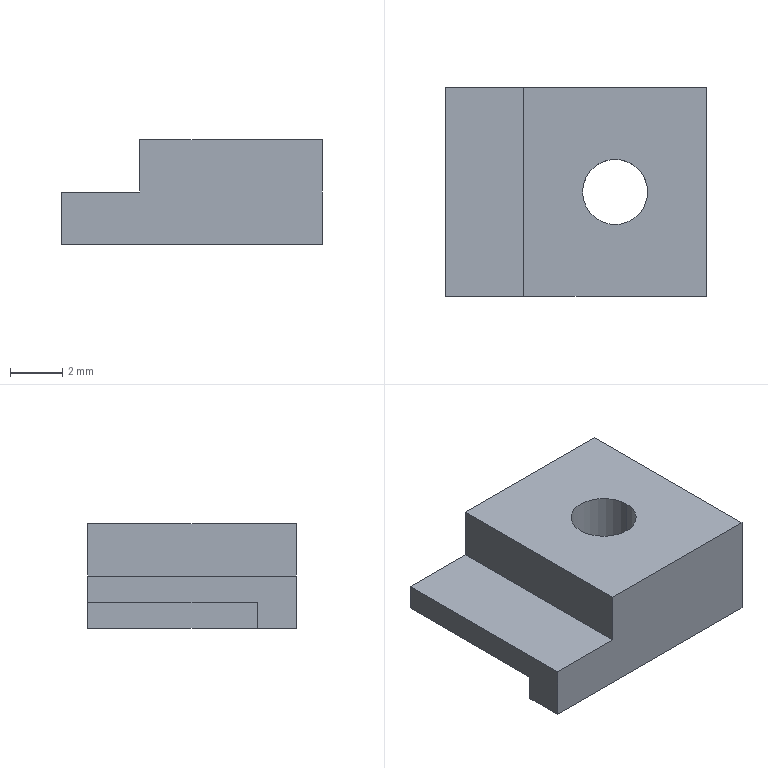Part | SolidWorks | features ICE 4, Extrusion 1, HoleWzd 1, MoveFace 1 | 1 solid | 13 faces | box 10 x 8 x 4 mm | volume 226.365 mm3 | plane 11 | cylinder 2 | commonest cylinder face diameters 2.5 x2
STEP:
#1=CARTESIAN_POINT('',(7.25,-4.,0.));
#2=VERTEX_POINT('',#1);
#3=CARTESIAN_POINT('',(9.75,-4.,0.));
#4=VERTEX_POINT('',#3);
#5=CARTESIAN_POINT('',(8.5,-4.,0.));
#6=DIRECTION('',(0.,0.,1.));
#7=DIRECTION('',(1.,0.,0.));
#8=AXIS2_PLACEMENT_3D('',#5,#6,#7);
#9=CIRCLE('',#8,1.25);
#10=EDGE_CURVE('',#2,#4,#9,.T.);
#11=ORIENTED_EDGE('',*,*,#10,.F.);
#12=CARTESIAN_POINT('',(7.25,-4.,4.));
#13=VERTEX_POINT('',#12);
#14=CARTESIAN_POINT('',(7.25,-4.,4.));
#15=DIRECTION('',(0.,0.,1.));
#16=VECTOR('',#15,1000.);
#17=LINE('',#14,#16);
#18=EDGE_CURVE('',#2,#13,#17,.T.);
#19=ORIENTED_EDGE('',*,*,#18,.T.);
#20=CARTESIAN_POINT('',(9.75,-4.,4.));
#21=VERTEX_POINT('',#20);
#22=CARTESIAN_POINT('',(8.5,-4.,4.));
#23=DIRECTION('',(0.,0.,1.));
#24=DIRECTION('',(1.,0.,0.));
#25=AXIS2_PLACEMENT_3D('',#22,#23,#24);
#26=CIRCLE('',#25,1.25);
#27=EDGE_CURVE('',#13,#21,#26,.T.);
#28=ORIENTED_EDGE('',*,*,#27,.T.);
#29=CARTESIAN_POINT('',(9.75,-4.,4.));
#30=DIRECTION('',(0.,0.,1.));
#31=VECTOR('',#30,1000.);
#32=LINE('',#29,#31);
#33=EDGE_CURVE('',#4,#21,#32,.T.);
#34=ORIENTED_EDGE('',*,*,#33,.F.);
#35=EDGE_LOOP('',(#11,#19,#28,#34));
#36=FACE_OUTER_BOUND('',#35,.T.);
#37=CARTESIAN_POINT('',(8.5,-4.,4.));
#38=DIRECTION('',(0.,0.,1.));
#39=DIRECTION('',(1.,0.,0.));
#40=AXIS2_PLACEMENT_3D('',#37,#38,#39);
#41=CYLINDRICAL_SURFACE('',#40,1.25);
#42=ADVANCED_FACE('',(#36),#41,.F.);
#43=CARTESIAN_POINT('',(2.,-8.,2.));
#44=VERTEX_POINT('',#43);
#45=CARTESIAN_POINT('',(5.,-8.,2.));
#46=VERTEX_POINT('',#45);
#47=CARTESIAN_POINT('',(0.,-8.,2.));
#48=DIRECTION('',(1.,0.,0.));
#49=VECTOR('',#48,1000.);
#50=LINE('',#47,#49);
#51=EDGE_CURVE('',#44,#46,#50,.T.);
#52=ORIENTED_EDGE('',*,*,#51,.F.);
#53=CARTESIAN_POINT('',(2.,-8.,0.));
#54=VERTEX_POINT('',#53);
#55=CARTESIAN_POINT('',(2.,-8.,7.));
#56=DIRECTION('',(0.,0.,-1.));
#57=VECTOR('',#56,1000.);
#58=LINE('',#55,#57);
#59=EDGE_CURVE('',#44,#54,#58,.T.);
#60=ORIENTED_EDGE('',*,*,#59,.T.);
#61=CARTESIAN_POINT('',(12.,-8.,0.));
#62=VERTEX_POINT('',#61);
#63=CARTESIAN_POINT('',(0.,-8.,0.));
#64=DIRECTION('',(1.,0.,0.));
#65=VECTOR('',#64,1000.);
#66=LINE('',#63,#65);
#67=EDGE_CURVE('',#54,#62,#66,.T.);
#68=ORIENTED_EDGE('',*,*,#67,.T.);
#69=CARTESIAN_POINT('',(12.,-8.,4.));
#70=VERTEX_POINT('',#69);
#71=CARTESIAN_POINT('',(12.,-8.,2.));
#72=DIRECTION('',(0.,0.,-1.));
#73=VECTOR('',#72,1000.);
#74=LINE('',#71,#73);
#75=EDGE_CURVE('',#70,#62,#74,.T.);
#76=ORIENTED_EDGE('',*,*,#75,.F.);
#77=CARTESIAN_POINT('',(5.,-8.,4.));
#78=VERTEX_POINT('',#77);
#79=CARTESIAN_POINT('',(12.,-8.,4.));
#80=DIRECTION('',(1.,0.,0.));
#81=VECTOR('',#80,1000.);
#82=LINE('',#79,#81);
#83=EDGE_CURVE('',#78,#70,#82,.T.);
#84=ORIENTED_EDGE('',*,*,#83,.F.);
#85=CARTESIAN_POINT('',(5.,-8.,4.));
#86=DIRECTION('',(0.,0.,-1.));
#87=VECTOR('',#86,1000.);
#88=LINE('',#85,#87);
#89=EDGE_CURVE('',#78,#46,#88,.T.);
#90=ORIENTED_EDGE('',*,*,#89,.T.);
#91=EDGE_LOOP('',(#52,#60,#68,#76,#84,#90));
#92=FACE_OUTER_BOUND('',#91,.T.);
#93=CARTESIAN_POINT('',(0.,-8.,2.));
#94=DIRECTION('',(0.,1.,0.));
#95=DIRECTION('',(0.,0.,1.));
#96=AXIS2_PLACEMENT_3D('',#93,#94,#95);
#97=PLANE('',#96);
#98=ADVANCED_FACE('',(#92),#97,.F.);
#99=CARTESIAN_POINT('',(12.,0.,0.));
#100=VERTEX_POINT('',#99);
#101=CARTESIAN_POINT('',(12.,0.,0.));
#102=DIRECTION('',(0.,1.,0.));
#103=VECTOR('',#102,1000.);
#104=LINE('',#101,#103);
#105=EDGE_CURVE('',#62,#100,#104,.T.);
#106=ORIENTED_EDGE('',*,*,#105,.T.);
#107=CARTESIAN_POINT('',(12.,0.,4.));
#108=VERTEX_POINT('',#107);
#109=CARTESIAN_POINT('',(12.,0.,2.));
#110=DIRECTION('',(0.,0.,-1.));
#111=VECTOR('',#110,1000.);
#112=LINE('',#109,#111);
#113=EDGE_CURVE('',#108,#100,#112,.T.);
#114=ORIENTED_EDGE('',*,*,#113,.F.);
#115=CARTESIAN_POINT('',(12.,-8.,4.));
#116=DIRECTION('',(0.,1.,0.));
#117=VECTOR('',#116,1000.);
#118=LINE('',#115,#117);
#119=EDGE_CURVE('',#70,#108,#118,.T.);
#120=ORIENTED_EDGE('',*,*,#119,.F.);
#121=ORIENTED_EDGE('',*,*,#75,.T.);
#122=EDGE_LOOP('',(#106,#114,#120,#121));
#123=FACE_OUTER_BOUND('',#122,.T.);
#124=CARTESIAN_POINT('',(12.,0.,2.));
#125=DIRECTION('',(-1.,0.,0.));
#126=DIRECTION('',(0.,-1.,0.));
#127=AXIS2_PLACEMENT_3D('',#124,#125,#126);
#128=PLANE('',#127);
#129=ADVANCED_FACE('',(#123),#128,.F.);
#130=CARTESIAN_POINT('',(2.,0.,1.));
#131=VERTEX_POINT('',#130);
#132=CARTESIAN_POINT('',(6.,0.,1.));
#133=VERTEX_POINT('',#132);
#134=CARTESIAN_POINT('',(0.,0.,1.));
#135=DIRECTION('',(1.,0.,0.));
#136=VECTOR('',#135,1000.);
#137=LINE('',#134,#136);
#138=EDGE_CURVE('',#131,#133,#137,.T.);
#139=ORIENTED_EDGE('',*,*,#138,.F.);
#140=CARTESIAN_POINT('',(2.,0.,2.));
#141=VERTEX_POINT('',#140);
#142=CARTESIAN_POINT('',(2.,0.,7.));
#143=DIRECTION('',(0.,0.,-1.));
#144=VECTOR('',#143,1000.);
#145=LINE('',#142,#144);
#146=EDGE_CURVE('',#141,#131,#145,.T.);
#147=ORIENTED_EDGE('',*,*,#146,.F.);
#148=CARTESIAN_POINT('',(5.,0.,2.));
#149=VERTEX_POINT('',#148);
#150=CARTESIAN_POINT('',(0.,0.,2.));
#151=DIRECTION('',(-1.,0.,0.));
#152=VECTOR('',#151,1000.);
#153=LINE('',#150,#152);
#154=EDGE_CURVE('',#149,#141,#153,.T.);
#155=ORIENTED_EDGE('',*,*,#154,.F.);
#156=CARTESIAN_POINT('',(5.,0.,4.));
#157=VERTEX_POINT('',#156);
#158=CARTESIAN_POINT('',(5.,0.,4.));
#159=DIRECTION('',(0.,0.,-1.));
#160=VECTOR('',#159,1000.);
#161=LINE('',#158,#160);
#162=EDGE_CURVE('',#157,#149,#161,.T.);
#163=ORIENTED_EDGE('',*,*,#162,.F.);
#164=CARTESIAN_POINT('',(12.,0.,4.));
#165=DIRECTION('',(-1.,0.,0.));
#166=VECTOR('',#165,1000.);
#167=LINE('',#164,#166);
#168=EDGE_CURVE('',#108,#157,#167,.T.);
#169=ORIENTED_EDGE('',*,*,#168,.F.);
#170=ORIENTED_EDGE('',*,*,#113,.T.);
#171=CARTESIAN_POINT('',(6.,0.,0.));
#172=VERTEX_POINT('',#171);
#173=CARTESIAN_POINT('',(0.,0.,0.));
#174=DIRECTION('',(-1.,0.,0.));
#175=VECTOR('',#174,1000.);
#176=LINE('',#173,#175);
#177=EDGE_CURVE('',#100,#172,#176,.T.);
#178=ORIENTED_EDGE('',*,*,#177,.T.);
#179=CARTESIAN_POINT('',(6.,0.,2.));
#180=DIRECTION('',(0.,0.,1.));
#181=VECTOR('',#180,1000.);
#182=LINE('',#179,#181);
#183=EDGE_CURVE('',#172,#133,#182,.T.);
#184=ORIENTED_EDGE('',*,*,#183,.T.);
#185=EDGE_LOOP('',(#139,#147,#155,#163,#169,#170,#178,#184));
#186=FACE_OUTER_BOUND('',#185,.T.);
#187=CARTESIAN_POINT('',(0.,0.,2.));
#188=DIRECTION('',(0.,-1.,0.));
#189=DIRECTION('',(0.,0.,-1.));
#190=AXIS2_PLACEMENT_3D('',#187,#188,#189);
#191=PLANE('',#190);
#192=ADVANCED_FACE('',(#186),#191,.F.);
#193=CARTESIAN_POINT('',(2.,0.,2.));
#194=DIRECTION('',(0.,1.,0.));
#195=VECTOR('',#194,1000.);
#196=LINE('',#193,#195);
#197=EDGE_CURVE('',#44,#141,#196,.T.);
#198=ORIENTED_EDGE('',*,*,#197,.F.);
#199=ORIENTED_EDGE('',*,*,#51,.T.);
#200=CARTESIAN_POINT('',(5.,-8.,2.));
#201=DIRECTION('',(0.,-1.,0.));
#202=VECTOR('',#201,1000.);
#203=LINE('',#200,#202);
#204=EDGE_CURVE('',#149,#46,#203,.T.);
#205=ORIENTED_EDGE('',*,*,#204,.F.);
#206=ORIENTED_EDGE('',*,*,#154,.T.);
#207=EDGE_LOOP('',(#198,#199,#205,#206));
#208=FACE_OUTER_BOUND('',#207,.T.);
#209=CARTESIAN_POINT('',(0.,0.,2.));
#210=DIRECTION('',(0.,0.,1.));
#211=DIRECTION('',(1.,0.,0.));
#212=AXIS2_PLACEMENT_3D('',#209,#210,#211);
#213=PLANE('',#212);
#214=ADVANCED_FACE('',(#208),#213,.T.);
#215=CARTESIAN_POINT('',(8.5,-4.,0.));
#216=DIRECTION('',(0.,0.,1.));
#217=DIRECTION('',(1.,0.,0.));
#218=AXIS2_PLACEMENT_3D('',#215,#216,#217);
#219=CIRCLE('',#218,1.25);
#220=EDGE_CURVE('',#4,#2,#219,.T.);
#221=ORIENTED_EDGE('',*,*,#220,.T.);
#222=ORIENTED_EDGE('',*,*,#10,.T.);
#223=EDGE_LOOP('',(#221,#222));
#224=FACE_BOUND('',#223,.T.);
#225=ORIENTED_EDGE('',*,*,#67,.F.);
#226=CARTESIAN_POINT('',(2.,-6.5,0.));
#227=VERTEX_POINT('',#226);
#228=CARTESIAN_POINT('',(2.,-8.,0.));
#229=DIRECTION('',(0.,-1.,0.));
#230=VECTOR('',#229,1000.);
#231=LINE('',#228,#230);
#232=EDGE_CURVE('',#227,#54,#231,.T.);
#233=ORIENTED_EDGE('',*,*,#232,.F.);
#234=CARTESIAN_POINT('',(6.,-6.5,0.));
#235=VERTEX_POINT('',#234);
#236=CARTESIAN_POINT('',(6.,-6.5,0.));
#237=DIRECTION('',(-1.,0.,0.));
#238=VECTOR('',#237,1000.);
#239=LINE('',#236,#238);
#240=EDGE_CURVE('',#235,#227,#239,.T.);
#241=ORIENTED_EDGE('',*,*,#240,.F.);
#242=CARTESIAN_POINT('',(6.,0.,0.));
#243=DIRECTION('',(0.,1.,0.));
#244=VECTOR('',#243,1000.);
#245=LINE('',#242,#244);
#246=EDGE_CURVE('',#235,#172,#245,.T.);
#247=ORIENTED_EDGE('',*,*,#246,.T.);
#248=ORIENTED_EDGE('',*,*,#177,.F.);
#249=ORIENTED_EDGE('',*,*,#105,.F.);
#250=EDGE_LOOP('',(#225,#233,#241,#247,#248,#249));
#251=FACE_OUTER_BOUND('',#250,.T.);
#252=CARTESIAN_POINT('',(0.,0.,0.));
#253=DIRECTION('',(0.,0.,1.));
#254=DIRECTION('',(1.,0.,0.));
#255=AXIS2_PLACEMENT_3D('',#252,#253,#254);
#256=PLANE('',#255);
#257=ADVANCED_FACE('',(#224,#251),#256,.F.);
#258=ORIENTED_EDGE('',*,*,#204,.T.);
#259=ORIENTED_EDGE('',*,*,#89,.F.);
#260=CARTESIAN_POINT('',(5.,-8.,4.));
#261=DIRECTION('',(0.,-1.,0.));
#262=VECTOR('',#261,1000.);
#263=LINE('',#260,#262);
#264=EDGE_CURVE('',#157,#78,#263,.T.);
#265=ORIENTED_EDGE('',*,*,#264,.F.);
#266=ORIENTED_EDGE('',*,*,#162,.T.);
#267=EDGE_LOOP('',(#258,#259,#265,#266));
#268=FACE_OUTER_BOUND('',#267,.T.);
#269=CARTESIAN_POINT('',(5.,-8.,4.));
#270=DIRECTION('',(1.,0.,0.));
#271=DIRECTION('',(0.,0.,-1.));
#272=AXIS2_PLACEMENT_3D('',#269,#270,#271);
#273=PLANE('',#272);
#274=ADVANCED_FACE('',(#268),#273,.F.);
#275=CARTESIAN_POINT('',(8.5,-4.,4.));
#276=DIRECTION('',(0.,0.,1.));
#277=DIRECTION('',(1.,0.,0.));
#278=AXIS2_PLACEMENT_3D('',#275,#276,#277);
#279=CIRCLE('',#278,1.25);
#280=EDGE_CURVE('',#21,#13,#279,.T.);
#281=ORIENTED_EDGE('',*,*,#280,.F.);
#282=ORIENTED_EDGE('',*,*,#27,.F.);
#283=EDGE_LOOP('',(#281,#282));
#284=FACE_BOUND('',#283,.T.);
#285=ORIENTED_EDGE('',*,*,#119,.T.);
#286=ORIENTED_EDGE('',*,*,#168,.T.);
#287=ORIENTED_EDGE('',*,*,#264,.T.);
#288=ORIENTED_EDGE('',*,*,#83,.T.);
#289=EDGE_LOOP('',(#285,#286,#287,#288));
#290=FACE_OUTER_BOUND('',#289,.T.);
#291=CARTESIAN_POINT('',(0.,0.,4.));
#292=DIRECTION('',(0.,0.,1.));
#293=DIRECTION('',(1.,0.,0.));
#294=AXIS2_PLACEMENT_3D('',#291,#292,#293);
#295=PLANE('',#294);
#296=ADVANCED_FACE('',(#284,#290),#295,.T.);
#297=CARTESIAN_POINT('',(2.,-6.5,1.));
#298=VERTEX_POINT('',#297);
#299=CARTESIAN_POINT('',(2.,0.,1.));
#300=DIRECTION('',(0.,-1.,0.));
#301=VECTOR('',#300,1000.);
#302=LINE('',#299,#301);
#303=EDGE_CURVE('',#131,#298,#302,.T.);
#304=ORIENTED_EDGE('',*,*,#303,.F.);
#305=ORIENTED_EDGE('',*,*,#138,.T.);
#306=CARTESIAN_POINT('',(6.,-6.5,1.));
#307=VERTEX_POINT('',#306);
#308=CARTESIAN_POINT('',(6.,-4.,1.));
#309=DIRECTION('',(0.,-1.,0.));
#310=VECTOR('',#309,1000.);
#311=LINE('',#308,#310);
#312=EDGE_CURVE('',#133,#307,#311,.T.);
#313=ORIENTED_EDGE('',*,*,#312,.T.);
#314=CARTESIAN_POINT('',(6.,-6.5,1.));
#315=DIRECTION('',(-1.,0.,0.));
#316=VECTOR('',#315,1000.);
#317=LINE('',#314,#316);
#318=EDGE_CURVE('',#307,#298,#317,.T.);
#319=ORIENTED_EDGE('',*,*,#318,.T.);
#320=EDGE_LOOP('',(#304,#305,#313,#319));
#321=FACE_OUTER_BOUND('',#320,.T.);
#322=CARTESIAN_POINT('',(0.,0.,1.));
#323=DIRECTION('',(0.,0.,-1.));
#324=DIRECTION('',(-1.,0.,0.));
#325=AXIS2_PLACEMENT_3D('',#322,#323,#324);
#326=PLANE('',#325);
#327=ADVANCED_FACE('',(#321),#326,.T.);
#328=ORIENTED_EDGE('',*,*,#246,.F.);
#329=CARTESIAN_POINT('',(6.,-6.5,1.));
#330=DIRECTION('',(0.,0.,-1.));
#331=VECTOR('',#330,1000.);
#332=LINE('',#329,#331);
#333=EDGE_CURVE('',#307,#235,#332,.T.);
#334=ORIENTED_EDGE('',*,*,#333,.F.);
#335=ORIENTED_EDGE('',*,*,#312,.F.);
#336=ORIENTED_EDGE('',*,*,#183,.F.);
#337=EDGE_LOOP('',(#328,#334,#335,#336));
#338=FACE_OUTER_BOUND('',#337,.T.);
#339=CARTESIAN_POINT('',(6.,-4.,1.));
#340=DIRECTION('',(1.,0.,0.));
#341=DIRECTION('',(0.,0.,-1.));
#342=AXIS2_PLACEMENT_3D('',#339,#340,#341);
#343=PLANE('',#342);
#344=ADVANCED_FACE('',(#338),#343,.F.);
#345=ORIENTED_EDGE('',*,*,#240,.T.);
#346=CARTESIAN_POINT('',(2.,-6.5,1.));
#347=DIRECTION('',(0.,0.,1.));
#348=VECTOR('',#347,1000.);
#349=LINE('',#346,#348);
#350=EDGE_CURVE('',#227,#298,#349,.T.);
#351=ORIENTED_EDGE('',*,*,#350,.T.);
#352=ORIENTED_EDGE('',*,*,#318,.F.);
#353=ORIENTED_EDGE('',*,*,#333,.T.);
#354=EDGE_LOOP('',(#345,#351,#352,#353));
#355=FACE_OUTER_BOUND('',#354,.T.);
#356=CARTESIAN_POINT('',(6.,-6.5,1.));
#357=DIRECTION('',(0.,-1.,0.));
#358=DIRECTION('',(0.,0.,-1.));
#359=AXIS2_PLACEMENT_3D('',#356,#357,#358);
#360=PLANE('',#359);
#361=ADVANCED_FACE('',(#355),#360,.F.);
#362=ORIENTED_EDGE('',*,*,#197,.T.);
#363=ORIENTED_EDGE('',*,*,#146,.T.);
#364=ORIENTED_EDGE('',*,*,#303,.T.);
#365=ORIENTED_EDGE('',*,*,#350,.F.);
#366=ORIENTED_EDGE('',*,*,#232,.T.);
#367=ORIENTED_EDGE('',*,*,#59,.F.);
#368=EDGE_LOOP('',(#362,#363,#364,#365,#366,#367));
#369=FACE_OUTER_BOUND('',#368,.T.);
#370=CARTESIAN_POINT('',(2.,-8.,7.));
#371=DIRECTION('',(1.,0.,0.));
#372=DIRECTION('',(0.,0.,-1.));
#373=AXIS2_PLACEMENT_3D('',#370,#371,#372);
#374=PLANE('',#373);
#375=ADVANCED_FACE('',(#369),#374,.F.);
#376=ORIENTED_EDGE('',*,*,#18,.F.);
#377=ORIENTED_EDGE('',*,*,#220,.F.);
#378=ORIENTED_EDGE('',*,*,#33,.T.);
#379=ORIENTED_EDGE('',*,*,#280,.T.);
#380=EDGE_LOOP('',(#376,#377,#378,#379));
#381=FACE_OUTER_BOUND('',#380,.T.);
#382=CARTESIAN_POINT('',(8.5,-4.,4.));
#383=DIRECTION('',(0.,0.,1.));
#384=DIRECTION('',(1.,0.,0.));
#385=AXIS2_PLACEMENT_3D('',#382,#383,#384);
#386=CYLINDRICAL_SURFACE('',#385,1.25);
#387=ADVANCED_FACE('',(#381),#386,.F.);
#388=CLOSED_SHELL('',(#42,#98,#129,#192,#214,#257,#274,#296,#327,#344,#361,#375,#387));
#389=MANIFOLD_SOLID_BREP('',#388);
#390=CARTESIAN_POINT('',(0.,0.,0.));
#391=DIRECTION('',(0.,0.,1.));
#392=DIRECTION('',(1.,0.,0.));
#393=AXIS2_PLACEMENT_3D('',#390,#391,#392);
#394=(LENGTH_UNIT()NAMED_UNIT(*)SI_UNIT(.MILLI.,.METRE.));
#395=UNCERTAINTY_MEASURE_WITH_UNIT(LENGTH_MEASURE(0.00001),#394,'','');
#396=(NAMED_UNIT(*)PLANE_ANGLE_UNIT()SI_UNIT($,.RADIAN.));
#397=(NAMED_UNIT(*)SI_UNIT($,.STERADIAN.)SOLID_ANGLE_UNIT());
#398=(GEOMETRIC_REPRESENTATION_CONTEXT(3)GLOBAL_UNCERTAINTY_ASSIGNED_CONTEXT((#395))GLOBAL_UNIT_ASSIGNED_CONTEXT((#394,#396,#397))REPRESENTATION_CONTEXT('',''));
#399=ADVANCED_BREP_SHAPE_REPRESENTATION('',(#389,#393),#398);